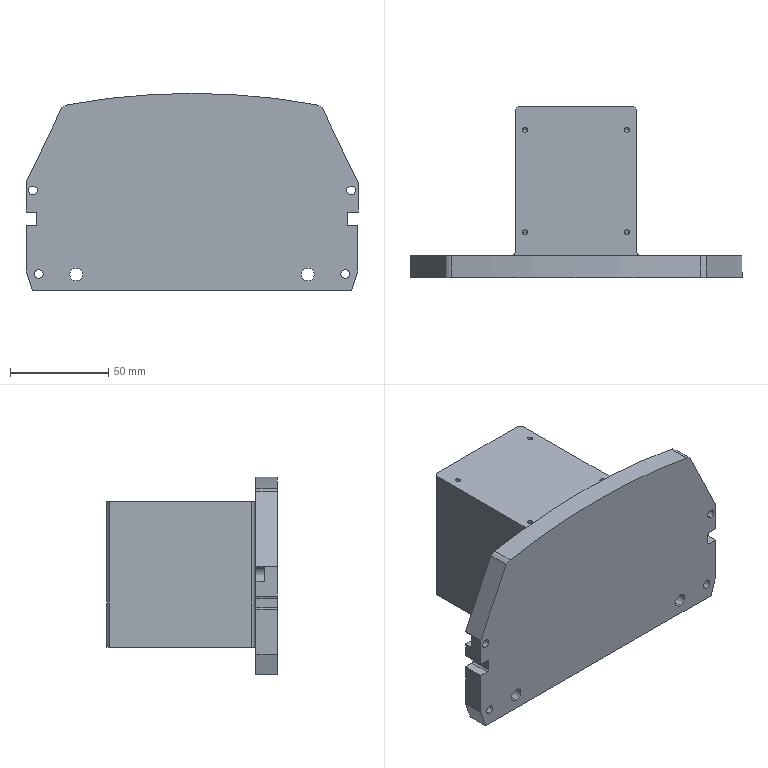Part | STEP file | 复件 FHB175-003^FHB175S-PRW-P40(马达RightUpper折-400W伺服电机) | 1 solid | 97 faces | box 169 x 87 x 100.4 mm | volume 517435 mm3 | cylinder 47 | plane 34 | cone 16 | commonest cylinder face diameters 2.5 x16 4.5 x8 7.5 x6 2 x4 6.6 x4 10.5 x4